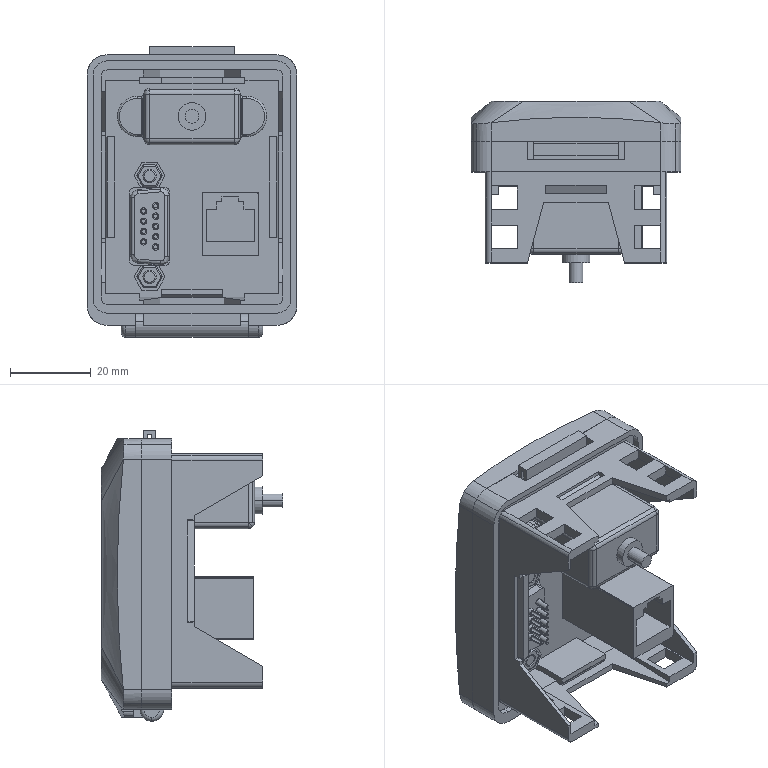Part | SolidWorks | features BaseBody 10 | 10 solids | 1001 faces | box 52 x 45 x 71.95 mm | volume 42694 mm3 | plane 540 | cylinder 323 | cone 76 | sphere 26 | spline 20 | torus 16 | commonest cylinder face diameters 1 x128 3 x46 4 x20 1.6 x18 10 x18 2 x16